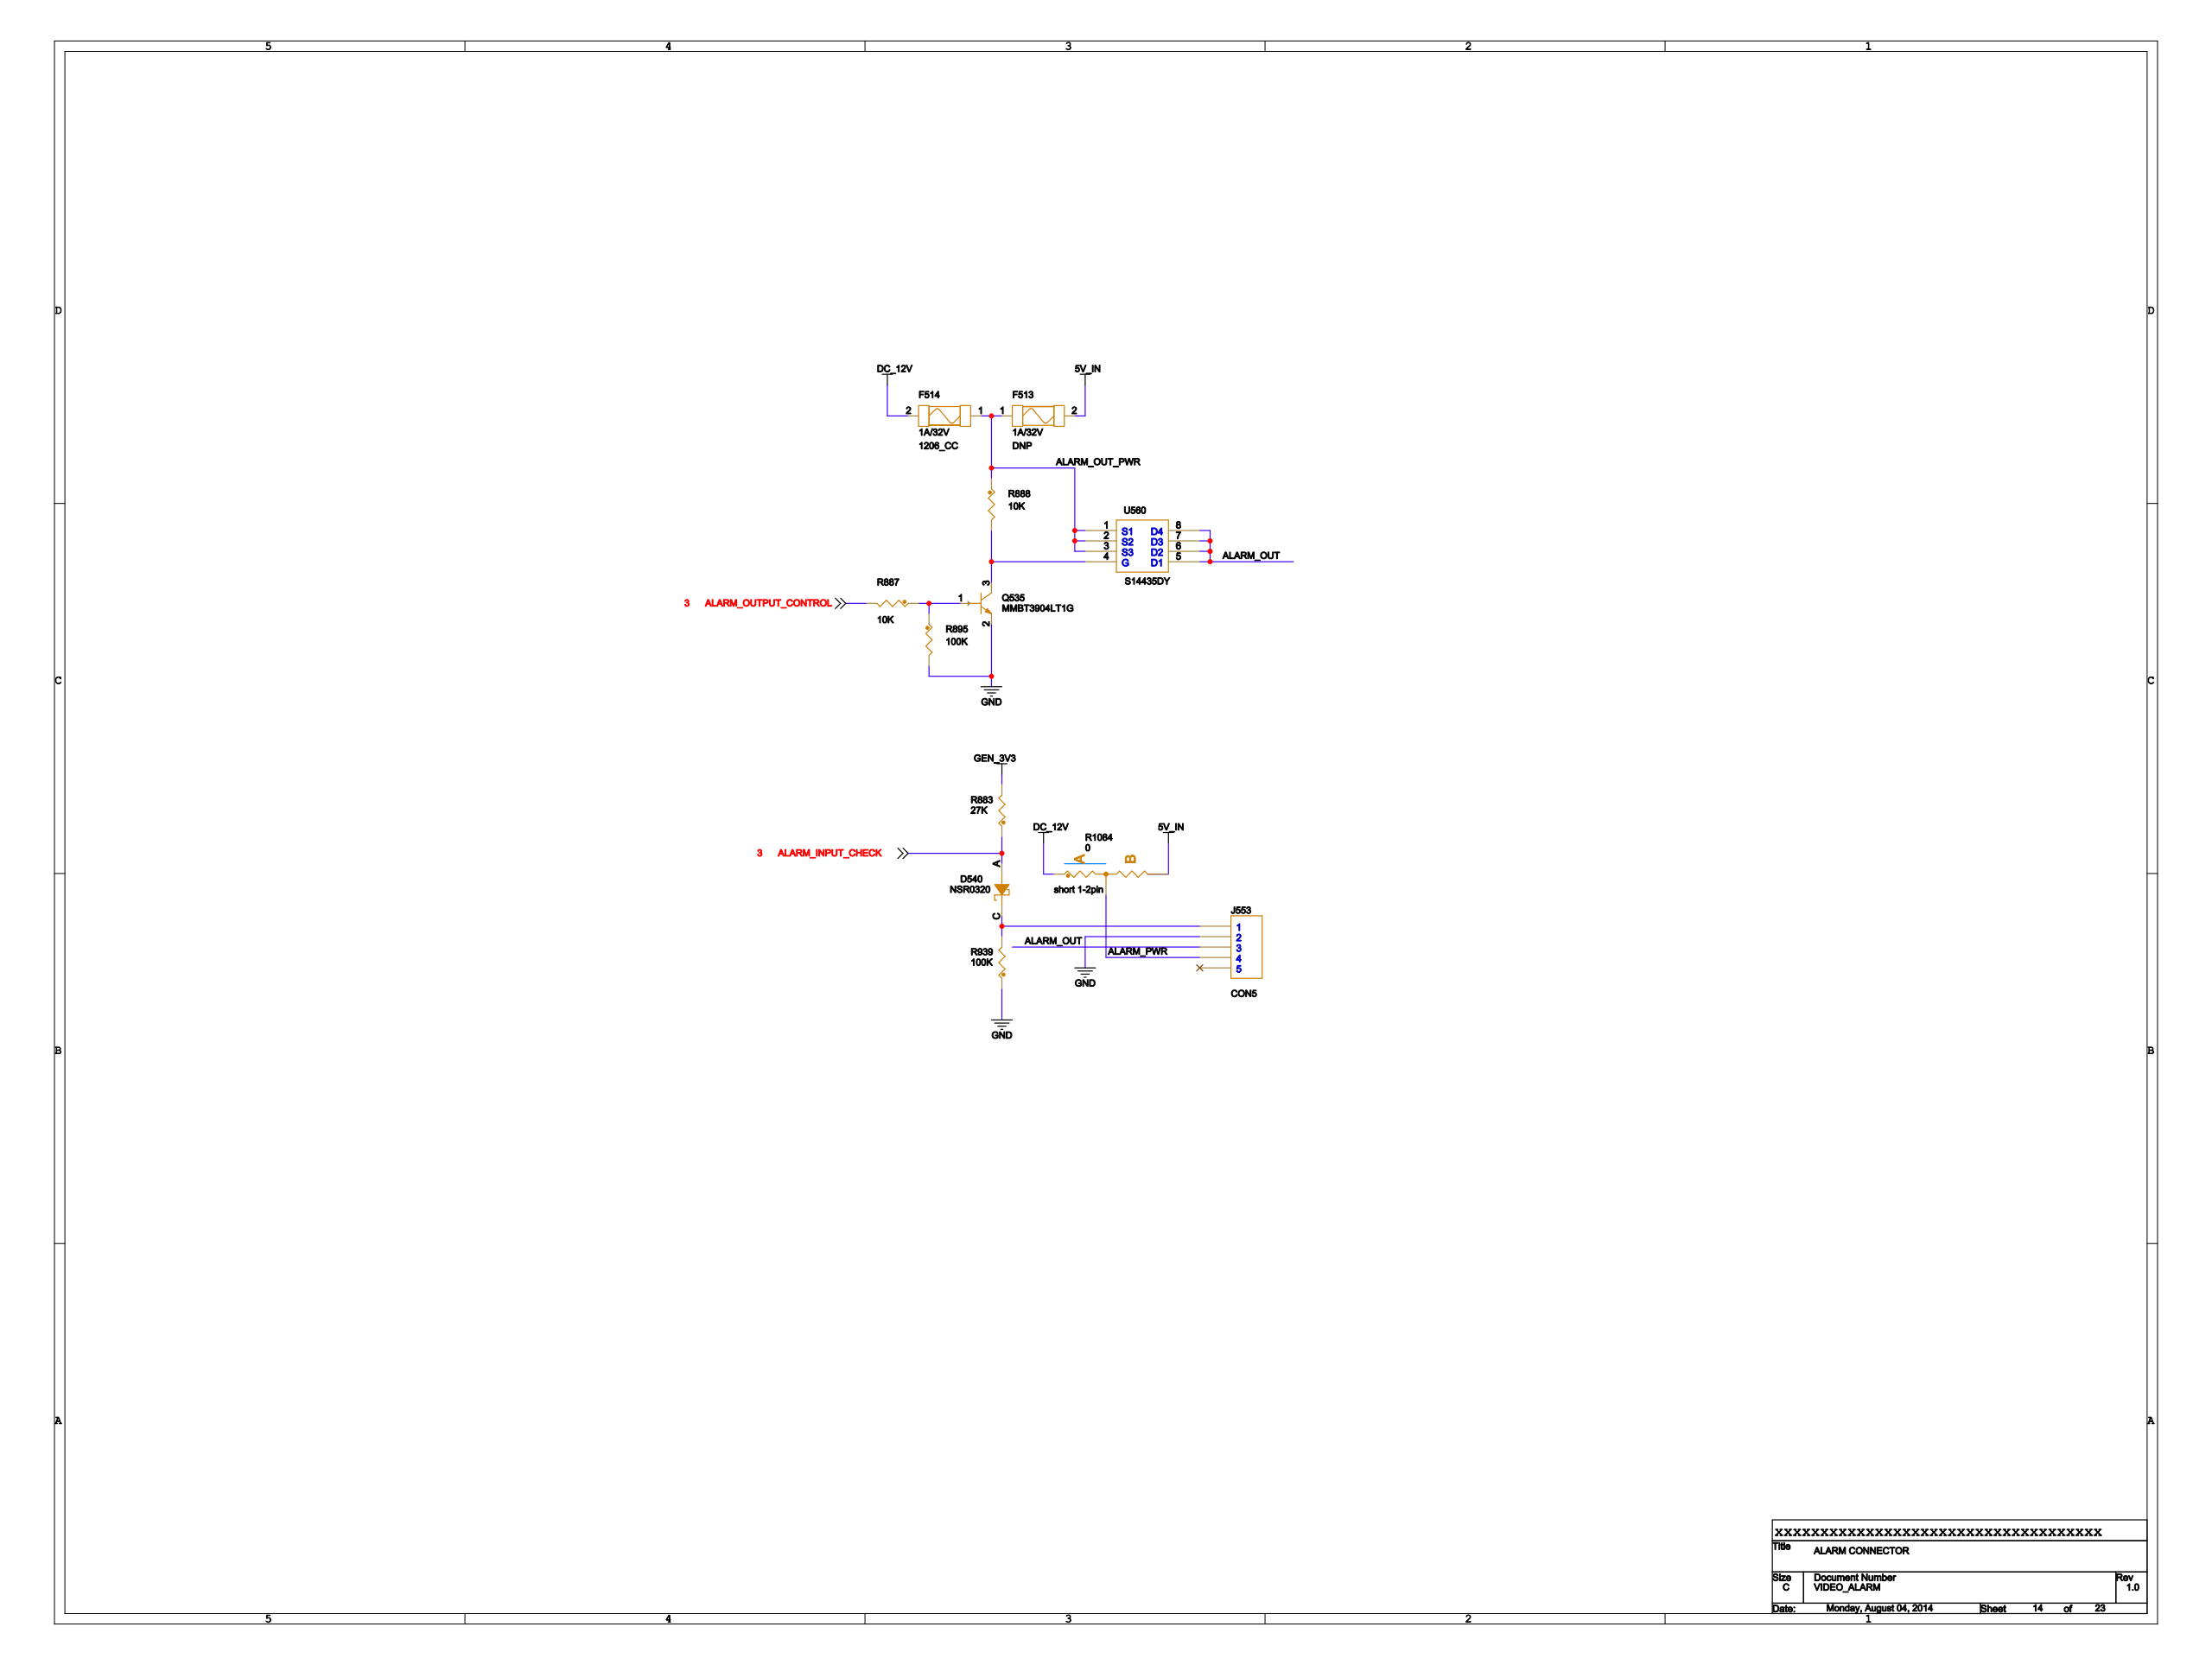Circuit board | Cadence Allegro | 994 parts | 728 nets | one sheet of the schematic
Parts on this sheet (reference | value | footprint):
D540 | NSR0320 | SOD323
F513 | 1A/32V | 1206_CC
F514 | 1A/32V | 1206_CC
J553 | CON5 | CON5
Q535 | MMBT3904LT1G | SOT23
R883 | 27K | 0603_CC
R887 | 10K | 0603_CC
R888 | 10K | 0603_CC
R895 | 100K | 0603_CC
R939 | 100K | 0603_CC
R1084 | 0 | R1206-X2
U560 | S14435DY | SI4435DY
Nets of these parts (net: part-pin ...):
GND: J553-2 Q535-2 R895-2 R939-1
GEN_3V3: R883-2
DC_12V: F514-2 R1084-1
ALARM_PWR: J553-4 R1084-2
5V_IN: F513-2 R1084-3
N22491903: D540-C J553-1 R939-2
ALARM_OUT: J553-3 U560-5 U560-6 U560-7 U560-8
ALARM_INPUT_CHECK: D540-A R883-1
N22491588: Q535-1 R887-1 R895-1
ALARM_OUT_PWR: F513-1 F514-1 R888-1 U560-1 U560-2 U560-3
N22491563: Q535-3 R888-2 U560-4
ALARM_OUTPUT_CONTROL: R887-2